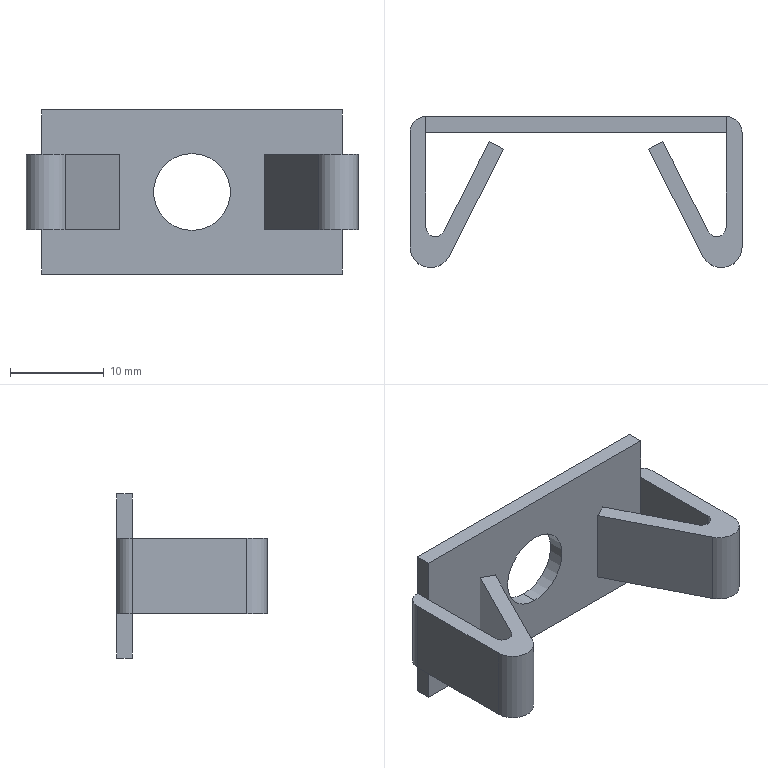Part | SolidWorks | features BaseBody 1 | 1 solid | 30 faces | box 35.4 x 16.108 x 17.5 mm | volume 1712 mm3 | plane 22 | cylinder 8 | commonest cylinder face diameters 2 x2 3.4 x2 4.4 x2 8.2 x2
STEP:
#1=CARTESIAN_POINT('',(0.,-1.7,-4.1));
#2=VERTEX_POINT('',#1);
#3=CARTESIAN_POINT('',(0.,-1.7,4.1));
#4=VERTEX_POINT('',#3);
#5=CARTESIAN_POINT('',(0.,-1.7,0.));
#6=DIRECTION('',(0.,1.,0.));
#7=DIRECTION('',(0.,0.,1.));
#8=AXIS2_PLACEMENT_3D('',#5,#6,#7);
#9=CIRCLE('',#8,4.1);
#10=EDGE_CURVE('',#2,#4,#9,.T.);
#11=ORIENTED_EDGE('',*,*,#10,.F.);
#12=CARTESIAN_POINT('',(0.,0.,-4.1));
#13=VERTEX_POINT('',#12);
#14=CARTESIAN_POINT('',(0.,-1.7,-4.1));
#15=DIRECTION('',(0.,1.,0.));
#16=VECTOR('',#15,1000.);
#17=LINE('',#14,#16);
#18=EDGE_CURVE('',#2,#13,#17,.T.);
#19=ORIENTED_EDGE('',*,*,#18,.T.);
#20=CARTESIAN_POINT('',(0.,0.,4.1));
#21=VERTEX_POINT('',#20);
#22=CARTESIAN_POINT('',(0.,0.,0.));
#23=DIRECTION('',(0.,1.,0.));
#24=DIRECTION('',(0.,0.,1.));
#25=AXIS2_PLACEMENT_3D('',#22,#23,#24);
#26=CIRCLE('',#25,4.1);
#27=EDGE_CURVE('',#13,#21,#26,.T.);
#28=ORIENTED_EDGE('',*,*,#27,.T.);
#29=CARTESIAN_POINT('',(0.,-1.7,4.1));
#30=DIRECTION('',(0.,1.,0.));
#31=VECTOR('',#30,1000.);
#32=LINE('',#29,#31);
#33=EDGE_CURVE('',#4,#21,#32,.T.);
#34=ORIENTED_EDGE('',*,*,#33,.F.);
#35=EDGE_LOOP('',(#11,#19,#28,#34));
#36=FACE_OUTER_BOUND('',#35,.T.);
#37=CARTESIAN_POINT('',(0.,-1.7,0.));
#38=DIRECTION('',(0.,1.,0.));
#39=DIRECTION('',(0.,0.,1.));
#40=AXIS2_PLACEMENT_3D('',#37,#38,#39);
#41=CYLINDRICAL_SURFACE('',#40,4.1);
#42=ADVANCED_FACE('',(#36),#41,.F.);
#43=CARTESIAN_POINT('',(-16.,0.,-4.));
#44=VERTEX_POINT('',#43);
#45=CARTESIAN_POINT('',(-16.,0.,-8.75));
#46=VERTEX_POINT('',#45);
#47=CARTESIAN_POINT('',(-16.,0.,8.75));
#48=DIRECTION('',(0.,0.,-1.));
#49=VECTOR('',#48,1000.);
#50=LINE('',#47,#49);
#51=EDGE_CURVE('',#44,#46,#50,.T.);
#52=ORIENTED_EDGE('',*,*,#51,.F.);
#53=CARTESIAN_POINT('',(-16.,0.,4.));
#54=VERTEX_POINT('',#53);
#55=CARTESIAN_POINT('',(-16.,0.,8.75));
#56=DIRECTION('',(0.,0.,-1.));
#57=VECTOR('',#56,1000.);
#58=LINE('',#55,#57);
#59=EDGE_CURVE('',#54,#44,#58,.T.);
#60=ORIENTED_EDGE('',*,*,#59,.F.);
#61=CARTESIAN_POINT('',(-16.,0.,8.75));
#62=VERTEX_POINT('',#61);
#63=CARTESIAN_POINT('',(-16.,0.,8.75));
#64=DIRECTION('',(0.,0.,-1.));
#65=VECTOR('',#64,1000.);
#66=LINE('',#63,#65);
#67=EDGE_CURVE('',#62,#54,#66,.T.);
#68=ORIENTED_EDGE('',*,*,#67,.F.);
#69=CARTESIAN_POINT('',(16.,0.,8.75));
#70=VERTEX_POINT('',#69);
#71=CARTESIAN_POINT('',(16.,0.,8.75));
#72=DIRECTION('',(-1.,0.,0.));
#73=VECTOR('',#72,1000.);
#74=LINE('',#71,#73);
#75=EDGE_CURVE('',#70,#62,#74,.T.);
#76=ORIENTED_EDGE('',*,*,#75,.F.);
#77=CARTESIAN_POINT('',(16.,0.,4.));
#78=VERTEX_POINT('',#77);
#79=CARTESIAN_POINT('',(16.,0.,8.75));
#80=DIRECTION('',(0.,0.,1.));
#81=VECTOR('',#80,1000.);
#82=LINE('',#79,#81);
#83=EDGE_CURVE('',#78,#70,#82,.T.);
#84=ORIENTED_EDGE('',*,*,#83,.F.);
#85=CARTESIAN_POINT('',(16.,0.,-4.));
#86=VERTEX_POINT('',#85);
#87=CARTESIAN_POINT('',(16.,0.,8.75));
#88=DIRECTION('',(0.,0.,1.));
#89=VECTOR('',#88,1000.);
#90=LINE('',#87,#89);
#91=EDGE_CURVE('',#86,#78,#90,.T.);
#92=ORIENTED_EDGE('',*,*,#91,.F.);
#93=CARTESIAN_POINT('',(16.,0.,-8.75));
#94=VERTEX_POINT('',#93);
#95=CARTESIAN_POINT('',(16.,0.,8.75));
#96=DIRECTION('',(0.,0.,1.));
#97=VECTOR('',#96,1000.);
#98=LINE('',#95,#97);
#99=EDGE_CURVE('',#94,#86,#98,.T.);
#100=ORIENTED_EDGE('',*,*,#99,.F.);
#101=CARTESIAN_POINT('',(16.,0.,-8.75));
#102=DIRECTION('',(1.,0.,0.));
#103=VECTOR('',#102,1000.);
#104=LINE('',#101,#103);
#105=EDGE_CURVE('',#46,#94,#104,.T.);
#106=ORIENTED_EDGE('',*,*,#105,.F.);
#107=EDGE_LOOP('',(#52,#60,#68,#76,#84,#92,#100,#106));
#108=FACE_OUTER_BOUND('',#107,.T.);
#109=CARTESIAN_POINT('',(0.,0.,0.));
#110=DIRECTION('',(0.,1.,0.));
#111=DIRECTION('',(0.,0.,1.));
#112=AXIS2_PLACEMENT_3D('',#109,#110,#111);
#113=CIRCLE('',#112,4.1);
#114=EDGE_CURVE('',#21,#13,#113,.T.);
#115=ORIENTED_EDGE('',*,*,#114,.F.);
#116=ORIENTED_EDGE('',*,*,#27,.F.);
#117=EDGE_LOOP('',(#115,#116));
#118=FACE_BOUND('',#117,.T.);
#119=CARTESIAN_POINT('',(16.,0.,8.75));
#120=DIRECTION('',(0.,-1.,0.));
#121=DIRECTION('',(0.,0.,-1.));
#122=AXIS2_PLACEMENT_3D('',#119,#120,#121);
#123=PLANE('',#122);
#124=ADVANCED_FACE('',(#108,#118),#123,.F.);
#125=ORIENTED_EDGE('',*,*,#105,.T.);
#126=CARTESIAN_POINT('',(16.,-1.7,-8.75));
#127=VERTEX_POINT('',#126);
#128=CARTESIAN_POINT('',(16.,0.,-8.75));
#129=DIRECTION('',(0.,1.,0.));
#130=VECTOR('',#129,1000.);
#131=LINE('',#128,#130);
#132=EDGE_CURVE('',#127,#94,#131,.T.);
#133=ORIENTED_EDGE('',*,*,#132,.F.);
#134=CARTESIAN_POINT('',(-16.,-1.7,-8.75));
#135=VERTEX_POINT('',#134);
#136=CARTESIAN_POINT('',(0.,-1.7,-8.75));
#137=DIRECTION('',(1.,0.,0.));
#138=VECTOR('',#137,1000.);
#139=LINE('',#136,#138);
#140=EDGE_CURVE('',#135,#127,#139,.T.);
#141=ORIENTED_EDGE('',*,*,#140,.F.);
#142=CARTESIAN_POINT('',(-16.,0.,-8.75));
#143=DIRECTION('',(0.,-1.,0.));
#144=VECTOR('',#143,1000.);
#145=LINE('',#142,#144);
#146=EDGE_CURVE('',#46,#135,#145,.T.);
#147=ORIENTED_EDGE('',*,*,#146,.F.);
#148=EDGE_LOOP('',(#125,#133,#141,#147));
#149=FACE_OUTER_BOUND('',#148,.T.);
#150=CARTESIAN_POINT('',(0.,0.,-8.75));
#151=DIRECTION('',(0.,0.,1.));
#152=DIRECTION('',(1.,0.,0.));
#153=AXIS2_PLACEMENT_3D('',#150,#151,#152);
#154=PLANE('',#153);
#155=ADVANCED_FACE('',(#149),#154,.F.);
#156=ORIENTED_EDGE('',*,*,#51,.T.);
#157=ORIENTED_EDGE('',*,*,#146,.T.);
#158=CARTESIAN_POINT('',(-16.,-1.7,-4.));
#159=VERTEX_POINT('',#158);
#160=CARTESIAN_POINT('',(-16.,-1.7,8.75));
#161=DIRECTION('',(0.,0.,-1.));
#162=VECTOR('',#161,1000.);
#163=LINE('',#160,#162);
#164=EDGE_CURVE('',#159,#135,#163,.T.);
#165=ORIENTED_EDGE('',*,*,#164,.F.);
#166=CARTESIAN_POINT('',(-16.,-1.7,-4.));
#167=DIRECTION('',(0.,1.,0.));
#168=VECTOR('',#167,1000.);
#169=LINE('',#166,#168);
#170=EDGE_CURVE('',#159,#44,#169,.T.);
#171=ORIENTED_EDGE('',*,*,#170,.T.);
#172=EDGE_LOOP('',(#156,#157,#165,#171));
#173=FACE_OUTER_BOUND('',#172,.T.);
#174=CARTESIAN_POINT('',(-16.,0.,8.75));
#175=DIRECTION('',(1.,0.,0.));
#176=DIRECTION('',(0.,0.,-1.));
#177=AXIS2_PLACEMENT_3D('',#174,#175,#176);
#178=PLANE('',#177);
#179=ADVANCED_FACE('',(#173),#178,.F.);
#180=CARTESIAN_POINT('',(-17.7,-1.7,4.));
#181=VERTEX_POINT('',#180);
#182=CARTESIAN_POINT('',(-16.,-1.7,4.));
#183=DIRECTION('',(0.,0.,-1.));
#184=DIRECTION('',(1.,0.,0.));
#185=AXIS2_PLACEMENT_3D('',#182,#183,#184);
#186=CIRCLE('',#185,1.7);
#187=EDGE_CURVE('',#181,#54,#186,.T.);
#188=ORIENTED_EDGE('',*,*,#187,.T.);
#189=ORIENTED_EDGE('',*,*,#59,.T.);
#190=CARTESIAN_POINT('',(-17.7,-1.7,-4.));
#191=VERTEX_POINT('',#190);
#192=CARTESIAN_POINT('',(-16.,-1.7,-4.));
#193=DIRECTION('',(0.,0.,1.));
#194=DIRECTION('',(1.,0.,0.));
#195=AXIS2_PLACEMENT_3D('',#192,#193,#194);
#196=CIRCLE('',#195,1.7);
#197=EDGE_CURVE('',#44,#191,#196,.T.);
#198=ORIENTED_EDGE('',*,*,#197,.T.);
#199=CARTESIAN_POINT('',(-17.7,-1.7,4.));
#200=DIRECTION('',(0.,0.,1.));
#201=VECTOR('',#200,1000.);
#202=LINE('',#199,#201);
#203=EDGE_CURVE('',#191,#181,#202,.T.);
#204=ORIENTED_EDGE('',*,*,#203,.T.);
#205=EDGE_LOOP('',(#188,#189,#198,#204));
#206=FACE_OUTER_BOUND('',#205,.T.);
#207=CARTESIAN_POINT('',(-16.,-1.7,4.));
#208=DIRECTION('',(0.,0.,1.));
#209=DIRECTION('',(1.,0.,0.));
#210=AXIS2_PLACEMENT_3D('',#207,#208,#209);
#211=CYLINDRICAL_SURFACE('',#210,1.7);
#212=ADVANCED_FACE('',(#206),#211,.T.);
#213=CARTESIAN_POINT('',(-16.,-1.7,4.));
#214=VERTEX_POINT('',#213);
#215=CARTESIAN_POINT('',(-16.,0.,4.));
#216=DIRECTION('',(0.,1.,0.));
#217=VECTOR('',#216,1000.);
#218=LINE('',#215,#217);
#219=EDGE_CURVE('',#214,#54,#218,.T.);
#220=ORIENTED_EDGE('',*,*,#219,.F.);
#221=CARTESIAN_POINT('',(-16.,-1.7,8.75));
#222=VERTEX_POINT('',#221);
#223=CARTESIAN_POINT('',(-16.,-1.7,8.75));
#224=DIRECTION('',(0.,0.,-1.));
#225=VECTOR('',#224,1000.);
#226=LINE('',#223,#225);
#227=EDGE_CURVE('',#222,#214,#226,.T.);
#228=ORIENTED_EDGE('',*,*,#227,.F.);
#229=CARTESIAN_POINT('',(-16.,0.,8.75));
#230=DIRECTION('',(0.,-1.,0.));
#231=VECTOR('',#230,1000.);
#232=LINE('',#229,#231);
#233=EDGE_CURVE('',#62,#222,#232,.T.);
#234=ORIENTED_EDGE('',*,*,#233,.F.);
#235=ORIENTED_EDGE('',*,*,#67,.T.);
#236=EDGE_LOOP('',(#220,#228,#234,#235));
#237=FACE_OUTER_BOUND('',#236,.T.);
#238=CARTESIAN_POINT('',(-16.,0.,8.75));
#239=DIRECTION('',(1.,0.,0.));
#240=DIRECTION('',(0.,0.,-1.));
#241=AXIS2_PLACEMENT_3D('',#238,#239,#240);
#242=PLANE('',#241);
#243=ADVANCED_FACE('',(#237),#242,.F.);
#244=CARTESIAN_POINT('',(16.,-1.7,8.75));
#245=VERTEX_POINT('',#244);
#246=CARTESIAN_POINT('',(16.,0.,8.75));
#247=DIRECTION('',(0.,1.,0.));
#248=VECTOR('',#247,1000.);
#249=LINE('',#246,#248);
#250=EDGE_CURVE('',#245,#70,#249,.T.);
#251=ORIENTED_EDGE('',*,*,#250,.T.);
#252=ORIENTED_EDGE('',*,*,#75,.T.);
#253=ORIENTED_EDGE('',*,*,#233,.T.);
#254=CARTESIAN_POINT('',(0.,-1.7,8.75));
#255=DIRECTION('',(1.,0.,0.));
#256=VECTOR('',#255,1000.);
#257=LINE('',#254,#256);
#258=EDGE_CURVE('',#222,#245,#257,.T.);
#259=ORIENTED_EDGE('',*,*,#258,.T.);
#260=EDGE_LOOP('',(#251,#252,#253,#259));
#261=FACE_OUTER_BOUND('',#260,.T.);
#262=CARTESIAN_POINT('',(0.,0.,8.75));
#263=DIRECTION('',(0.,0.,1.));
#264=DIRECTION('',(1.,0.,0.));
#265=AXIS2_PLACEMENT_3D('',#262,#263,#264);
#266=PLANE('',#265);
#267=ADVANCED_FACE('',(#261),#266,.T.);
#268=CARTESIAN_POINT('',(16.,-1.7,4.));
#269=VERTEX_POINT('',#268);
#270=CARTESIAN_POINT('',(16.,-13.908,4.));
#271=DIRECTION('',(0.,-1.,0.));
#272=VECTOR('',#271,1000.);
#273=LINE('',#270,#272);
#274=EDGE_CURVE('',#78,#269,#273,.T.);
#275=ORIENTED_EDGE('',*,*,#274,.F.);
#276=ORIENTED_EDGE('',*,*,#83,.T.);
#277=ORIENTED_EDGE('',*,*,#250,.F.);
#278=CARTESIAN_POINT('',(16.,-1.7,8.75));
#279=DIRECTION('',(0.,0.,1.));
#280=VECTOR('',#279,1000.);
#281=LINE('',#278,#280);
#282=EDGE_CURVE('',#269,#245,#281,.T.);
#283=ORIENTED_EDGE('',*,*,#282,.F.);
#284=EDGE_LOOP('',(#275,#276,#277,#283));
#285=FACE_OUTER_BOUND('',#284,.T.);
#286=CARTESIAN_POINT('',(16.,-1.7,8.75));
#287=DIRECTION('',(-1.,0.,0.));
#288=DIRECTION('',(0.,0.,1.));
#289=AXIS2_PLACEMENT_3D('',#286,#287,#288);
#290=PLANE('',#289);
#291=ADVANCED_FACE('',(#285),#290,.F.);
#292=CARTESIAN_POINT('',(17.7,-1.7,4.));
#293=VERTEX_POINT('',#292);
#294=CARTESIAN_POINT('',(16.,-1.7,4.));
#295=DIRECTION('',(0.,0.,-1.));
#296=DIRECTION('',(1.,0.,0.));
#297=AXIS2_PLACEMENT_3D('',#294,#295,#296);
#298=CIRCLE('',#297,1.7);
#299=EDGE_CURVE('',#78,#293,#298,.T.);
#300=ORIENTED_EDGE('',*,*,#299,.T.);
#301=CARTESIAN_POINT('',(17.7,-1.7,-4.));
#302=VERTEX_POINT('',#301);
#303=CARTESIAN_POINT('',(17.7,-1.7,4.));
#304=DIRECTION('',(0.,0.,-1.));
#305=VECTOR('',#304,1000.);
#306=LINE('',#303,#305);
#307=EDGE_CURVE('',#293,#302,#306,.T.);
#308=ORIENTED_EDGE('',*,*,#307,.T.);
#309=CARTESIAN_POINT('',(16.,-1.7,-4.));
#310=DIRECTION('',(0.,0.,1.));
#311=DIRECTION('',(1.,0.,0.));
#312=AXIS2_PLACEMENT_3D('',#309,#310,#311);
#313=CIRCLE('',#312,1.7);
#314=EDGE_CURVE('',#302,#86,#313,.T.);
#315=ORIENTED_EDGE('',*,*,#314,.T.);
#316=ORIENTED_EDGE('',*,*,#91,.T.);
#317=EDGE_LOOP('',(#300,#308,#315,#316));
#318=FACE_OUTER_BOUND('',#317,.T.);
#319=CARTESIAN_POINT('',(16.,-1.7,4.));
#320=DIRECTION('',(0.,0.,1.));
#321=DIRECTION('',(1.,0.,0.));
#322=AXIS2_PLACEMENT_3D('',#319,#320,#321);
#323=CYLINDRICAL_SURFACE('',#322,1.7);
#324=ADVANCED_FACE('',(#318),#323,.T.);
#325=CARTESIAN_POINT('',(16.,-1.7,-4.));
#326=VERTEX_POINT('',#325);
#327=CARTESIAN_POINT('',(16.,-1.7,8.75));
#328=DIRECTION('',(0.,0.,1.));
#329=VECTOR('',#328,1000.);
#330=LINE('',#327,#329);
#331=EDGE_CURVE('',#127,#326,#330,.T.);
#332=ORIENTED_EDGE('',*,*,#331,.F.);
#333=ORIENTED_EDGE('',*,*,#132,.T.);
#334=ORIENTED_EDGE('',*,*,#99,.T.);
#335=CARTESIAN_POINT('',(16.,-1.7,-4.));
#336=DIRECTION('',(0.,1.,0.));
#337=VECTOR('',#336,1000.);
#338=LINE('',#335,#337);
#339=EDGE_CURVE('',#326,#86,#338,.T.);
#340=ORIENTED_EDGE('',*,*,#339,.F.);
#341=EDGE_LOOP('',(#332,#333,#334,#340));
#342=FACE_OUTER_BOUND('',#341,.T.);
#343=CARTESIAN_POINT('',(16.,-1.7,8.75));
#344=DIRECTION('',(-1.,0.,0.));
#345=DIRECTION('',(0.,0.,1.));
#346=AXIS2_PLACEMENT_3D('',#343,#344,#345);
#347=PLANE('',#346);
#348=ADVANCED_FACE('',(#342),#347,.F.);
#349=ORIENTED_EDGE('',*,*,#18,.F.);
#350=CARTESIAN_POINT('',(0.,-1.7,0.));
#351=DIRECTION('',(0.,1.,0.));
#352=DIRECTION('',(0.,0.,1.));
#353=AXIS2_PLACEMENT_3D('',#350,#351,#352);
#354=CIRCLE('',#353,4.1);
#355=EDGE_CURVE('',#4,#2,#354,.T.);
#356=ORIENTED_EDGE('',*,*,#355,.F.);
#357=ORIENTED_EDGE('',*,*,#33,.T.);
#358=ORIENTED_EDGE('',*,*,#114,.T.);
#359=EDGE_LOOP('',(#349,#356,#357,#358));
#360=FACE_OUTER_BOUND('',#359,.T.);
#361=CARTESIAN_POINT('',(0.,-1.7,0.));
#362=DIRECTION('',(0.,1.,0.));
#363=DIRECTION('',(0.,0.,1.));
#364=AXIS2_PLACEMENT_3D('',#361,#362,#363);
#365=CYLINDRICAL_SURFACE('',#364,4.1);
#366=ADVANCED_FACE('',(#360),#365,.F.);
#367=ORIENTED_EDGE('',*,*,#331,.T.);
#368=CARTESIAN_POINT('',(16.,-1.7,8.75));
#369=DIRECTION('',(0.,0.,-1.));
#370=VECTOR('',#369,1000.);
#371=LINE('',#368,#370);
#372=EDGE_CURVE('',#269,#326,#371,.T.);
#373=ORIENTED_EDGE('',*,*,#372,.F.);
#374=ORIENTED_EDGE('',*,*,#282,.T.);
#375=ORIENTED_EDGE('',*,*,#258,.F.);
#376=ORIENTED_EDGE('',*,*,#227,.T.);
#377=CARTESIAN_POINT('',(-16.,-1.7,8.75));
#378=DIRECTION('',(0.,0.,1.));
#379=VECTOR('',#378,1000.);
#380=LINE('',#377,#379);
#381=EDGE_CURVE('',#159,#214,#380,.T.);
#382=ORIENTED_EDGE('',*,*,#381,.F.);
#383=ORIENTED_EDGE('',*,*,#164,.T.);
#384=ORIENTED_EDGE('',*,*,#140,.T.);
#385=EDGE_LOOP('',(#367,#373,#374,#375,#376,#382,#383,#384));
#386=FACE_OUTER_BOUND('',#385,.T.);
#387=ORIENTED_EDGE('',*,*,#355,.T.);
#388=ORIENTED_EDGE('',*,*,#10,.T.);
#389=EDGE_LOOP('',(#387,#388));
#390=FACE_BOUND('',#389,.T.);
#391=CARTESIAN_POINT('',(-16.,-1.7,8.75));
#392=DIRECTION('',(0.,1.,0.));
#393=DIRECTION('',(0.,0.,1.));
#394=AXIS2_PLACEMENT_3D('',#391,#392,#393);
#395=PLANE('',#394);
#396=ADVANCED_FACE('',(#386,#390),#395,.F.);
#397=CARTESIAN_POINT('',(-16.,-11.816,4.));
#398=VERTEX_POINT('',#397);
#399=CARTESIAN_POINT('',(-16.,-1.7,4.));
#400=DIRECTION('',(0.,1.,0.));
#401=VECTOR('',#400,1000.);
#402=LINE('',#399,#401);
#403=EDGE_CURVE('',#398,#214,#402,.T.);
#404=ORIENTED_EDGE('',*,*,#403,.T.);
#405=ORIENTED_EDGE('',*,*,#219,.T.);
#406=ORIENTED_EDGE('',*,*,#187,.F.);
#407=CARTESIAN_POINT('',(-17.7,-13.908,4.));
#408=VERTEX_POINT('',#407);
#409=CARTESIAN_POINT('',(-17.7,-1.7,4.));
#410=DIRECTION('',(0.,-1.,0.));
#411=VECTOR('',#410,1000.);
#412=LINE('',#409,#411);
#413=EDGE_CURVE('',#181,#408,#412,.T.);
#414=ORIENTED_EDGE('',*,*,#413,.T.);
#415=CARTESIAN_POINT('',(-13.538,-14.903,4.));
#416=VERTEX_POINT('',#415);
#417=CARTESIAN_POINT('',(-15.5,-13.908,4.));
#418=DIRECTION('',(0.,0.,1.));
#419=DIRECTION('',(1.,0.,0.));
#420=AXIS2_PLACEMENT_3D('',#417,#418,#419);
#421=CIRCLE('',#420,2.2);
#422=EDGE_CURVE('',#408,#416,#421,.T.);
#423=ORIENTED_EDGE('',*,*,#422,.T.);
#424=CARTESIAN_POINT('',(-7.741,-3.469,4.));
#425=VERTEX_POINT('',#424);
#426=CARTESIAN_POINT('',(-13.538,-14.903,4.));
#427=DIRECTION('',(0.4522,0.8919,0.));
#428=VECTOR('',#427,1000.);
#429=LINE('',#426,#428);
#430=EDGE_CURVE('',#416,#425,#429,.T.);
#431=ORIENTED_EDGE('',*,*,#430,.T.);
#432=CARTESIAN_POINT('',(-9.257,-2.7,4.));
#433=VERTEX_POINT('',#432);
#434=CARTESIAN_POINT('',(-7.741,-3.469,4.));
#435=DIRECTION('',(-0.8919,0.4522,0.));
#436=VECTOR('',#435,1000.);
#437=LINE('',#434,#436);
#438=EDGE_CURVE('',#425,#433,#437,.T.);
#439=ORIENTED_EDGE('',*,*,#438,.T.);
#440=CARTESIAN_POINT('',(-14.108,-12.268,4.));
#441=VERTEX_POINT('',#440);
#442=CARTESIAN_POINT('',(-9.257,-2.7,4.));
#443=DIRECTION('',(-0.4522,-0.8919,0.));
#444=VECTOR('',#443,1000.);
#445=LINE('',#442,#444);
#446=EDGE_CURVE('',#433,#441,#445,.T.);
#447=ORIENTED_EDGE('',*,*,#446,.T.);
#448=CARTESIAN_POINT('',(-15.,-11.816,4.));
#449=DIRECTION('',(0.,0.,-1.));
#450=DIRECTION('',(1.,0.,0.));
#451=AXIS2_PLACEMENT_3D('',#448,#449,#450);
#452=CIRCLE('',#451,1.);
#453=EDGE_CURVE('',#441,#398,#452,.T.);
#454=ORIENTED_EDGE('',*,*,#453,.T.);
#455=EDGE_LOOP('',(#404,#405,#406,#414,#423,#431,#439,#447,#454));
#456=FACE_OUTER_BOUND('',#455,.T.);
#457=CARTESIAN_POINT('',(-16.,-1.7,4.));
#458=DIRECTION('',(0.,0.,1.));
#459=DIRECTION('',(1.,0.,0.));
#460=AXIS2_PLACEMENT_3D('',#457,#458,#459);
#461=PLANE('',#460);
#462=ADVANCED_FACE('',(#456),#461,.T.);
#463=CARTESIAN_POINT('',(-17.7,-13.908,-4.));
#464=VERTEX_POINT('',#463);
#465=CARTESIAN_POINT('',(-17.7,-13.908,4.));
#466=DIRECTION('',(0.,0.,-1.));
#467=VECTOR('',#466,1000.);
#468=LINE('',#465,#467);
#469=EDGE_CURVE('',#408,#464,#468,.T.);
#470=ORIENTED_EDGE('',*,*,#469,.F.);
#471=ORIENTED_EDGE('',*,*,#413,.F.);
#472=ORIENTED_EDGE('',*,*,#203,.F.);
#473=CARTESIAN_POINT('',(-17.7,-1.7,-4.));
#474=DIRECTION('',(0.,1.,0.));
#475=VECTOR('',#474,1000.);
#476=LINE('',#473,#475);
#477=EDGE_CURVE('',#464,#191,#476,.T.);
#478=ORIENTED_EDGE('',*,*,#477,.F.);
#479=EDGE_LOOP('',(#470,#471,#472,#478));
#480=FACE_OUTER_BOUND('',#479,.T.);
#481=CARTESIAN_POINT('',(-17.7,-1.7,4.));
#482=DIRECTION('',(1.,0.,0.));
#483=DIRECTION('',(0.,0.,-1.));
#484=AXIS2_PLACEMENT_3D('',#481,#482,#483);
#485=PLANE('',#484);
#486=ADVANCED_FACE('',(#480),#485,.F.);
#487=ORIENTED_EDGE('',*,*,#170,.F.);
#488=CARTESIAN_POINT('',(-16.,-11.816,-4.));
#489=VERTEX_POINT('',#488);
#490=CARTESIAN_POINT('',(-16.,-1.7,-4.));
#491=DIRECTION('',(0.,1.,0.));
#492=VECTOR('',#491,1000.);
#493=LINE('',#490,#492);
#494=EDGE_CURVE('',#489,#159,#493,.T.);
#495=ORIENTED_EDGE('',*,*,#494,.F.);
#496=CARTESIAN_POINT('',(-14.108,-12.268,-4.));
#497=VERTEX_POINT('',#496);
#498=CARTESIAN_POINT('',(-15.,-11.816,-4.));
#499=DIRECTION('',(0.,0.,-1.));
#500=DIRECTION('',(1.,0.,0.));
#501=AXIS2_PLACEMENT_3D('',#498,#499,#500);
#502=CIRCLE('',#501,1.);
#503=EDGE_CURVE('',#497,#489,#502,.T.);
#504=ORIENTED_EDGE('',*,*,#503,.F.);
#505=CARTESIAN_POINT('',(-9.257,-2.7,-4.));
#506=VERTEX_POINT('',#505);
#507=CARTESIAN_POINT('',(-9.257,-2.7,-4.));
#508=DIRECTION('',(-0.4522,-0.8919,0.));
#509=VECTOR('',#508,1000.);
#510=LINE('',#507,#509);
#511=EDGE_CURVE('',#506,#497,#510,.T.);
#512=ORIENTED_EDGE('',*,*,#511,.F.);
#513=CARTESIAN_POINT('',(-7.741,-3.469,-4.));
#514=VERTEX_POINT('',#513);
#515=CARTESIAN_POINT('',(-7.741,-3.469,-4.));
#516=DIRECTION('',(0.8919,-0.4522,0.));
#517=VECTOR('',#516,1000.);
#518=LINE('',#515,#517);
#519=EDGE_CURVE('',#506,#514,#518,.T.);
#520=ORIENTED_EDGE('',*,*,#519,.T.);
#521=CARTESIAN_POINT('',(-13.538,-14.903,-4.));
#522=VERTEX_POINT('',#521);
#523=CARTESIAN_POINT('',(-13.538,-14.903,-4.));
#524=DIRECTION('',(0.4522,0.8919,0.));
#525=VECTOR('',#524,1000.);
#526=LINE('',#523,#525);
#527=EDGE_CURVE('',#522,#514,#526,.T.);
#528=ORIENTED_EDGE('',*,*,#527,.F.);
#529=CARTESIAN_POINT('',(-15.5,-13.908,-4.));
#530=DIRECTION('',(0.,0.,1.));
#531=DIRECTION('',(1.,0.,0.));
#532=AXIS2_PLACEMENT_3D('',#529,#530,#531);
#533=CIRCLE('',#532,2.2);
#534=EDGE_CURVE('',#464,#522,#533,.T.);
#535=ORIENTED_EDGE('',*,*,#534,.F.);
#536=ORIENTED_EDGE('',*,*,#477,.T.);
#537=ORIENTED_EDGE('',*,*,#197,.F.);
#538=EDGE_LOOP('',(#487,#495,#504,#512,#520,#528,#535,#536,#537));
#539=FACE_OUTER_BOUND('',#538,.T.);
#540=CARTESIAN_POINT('',(-16.,-1.7,-4.));
#541=DIRECTION('',(0.,0.,1.));
#542=DIRECTION('',(1.,0.,0.));
#543=AXIS2_PLACEMENT_3D('',#540,#541,#542);
#544=PLANE('',#543);
#545=ADVANCED_FACE('',(#539),#544,.F.);
#546=ORIENTED_EDGE('',*,*,#307,.F.);
#547=CARTESIAN_POINT('',(17.7,-13.908,4.));
#548=VERTEX_POINT('',#547);
#549=CARTESIAN_POINT('',(17.7,-13.908,4.));
#550=DIRECTION('',(0.,1.,0.));
#551=VECTOR('',#550,1000.);
#552=LINE('',#549,#551);
#553=EDGE_CURVE('',#548,#293,#552,.T.);
#554=ORIENTED_EDGE('',*,*,#553,.F.);
#555=CARTESIAN_POINT('',(17.7,-13.908,-4.));
#556=VERTEX_POINT('',#555);
#557=CARTESIAN_POINT('',(17.7,-13.908,4.));
#558=DIRECTION('',(0.,0.,1.));
#559=VECTOR('',#558,1000.);
#560=LINE('',#557,#559);
#561=EDGE_CURVE('',#556,#548,#560,.T.);
#562=ORIENTED_EDGE('',*,*,#561,.F.);
#563=CARTESIAN_POINT('',(17.7,-13.908,-4.));
#564=DIRECTION('',(0.,-1.,0.));
#565=VECTOR('',#564,1000.);
#566=LINE('',#563,#565);
#567=EDGE_CURVE('',#302,#556,#566,.T.);
#568=ORIENTED_EDGE('',*,*,#567,.F.);
#569=EDGE_LOOP('',(#546,#554,#562,#568));
#570=FACE_OUTER_BOUND('',#569,.T.);
#571=CARTESIAN_POINT('',(17.7,-13.908,4.));
#572=DIRECTION('',(-1.,0.,0.));
#573=DIRECTION('',(0.,0.,1.));
#574=AXIS2_PLACEMENT_3D('',#571,#572,#573);
#575=PLANE('',#574);
#576=ADVANCED_FACE('',(#570),#575,.F.);
#577=CARTESIAN_POINT('',(16.,-11.816,4.));
#578=VERTEX_POINT('',#577);
#579=CARTESIAN_POINT('',(14.108,-12.268,4.));
#580=VERTEX_POINT('',#579);
#581=CARTESIAN_POINT('',(15.,-11.816,4.));
#582=DIRECTION('',(0.,0.,-1.));
#583=DIRECTION('',(1.,0.,0.));
#584=AXIS2_PLACEMENT_3D('',#581,#582,#583);
#585=CIRCLE('',#584,1.);
#586=EDGE_CURVE('',#578,#580,#585,.T.);
#587=ORIENTED_EDGE('',*,*,#586,.T.);
#588=CARTESIAN_POINT('',(9.257,-2.7,4.));
#589=VERTEX_POINT('',#588);
#590=CARTESIAN_POINT('',(14.108,-12.268,4.));
#591=DIRECTION('',(-0.4522,0.8919,0.));
#592=VECTOR('',#591,1000.);
#593=LINE('',#590,#592);
#594=EDGE_CURVE('',#580,#589,#593,.T.);
#595=ORIENTED_EDGE('',*,*,#594,.T.);
#596=CARTESIAN_POINT('',(7.741,-3.469,4.));
#597=VERTEX_POINT('',#596);
#598=CARTESIAN_POINT('',(9.257,-2.7,4.));
#599=DIRECTION('',(-0.8919,-0.4522,0.));
#600=VECTOR('',#599,1000.);
#601=LINE('',#598,#600);
#602=EDGE_CURVE('',#589,#597,#601,.T.);
#603=ORIENTED_EDGE('',*,*,#602,.T.);
#604=CARTESIAN_POINT('',(13.538,-14.903,4.));
#605=VERTEX_POINT('',#604);
#606=CARTESIAN_POINT('',(7.741,-3.469,4.));
#607=DIRECTION('',(0.4522,-0.8919,0.));
#608=VECTOR('',#607,1000.);
#609=LINE('',#606,#608);
#610=EDGE_CURVE('',#597,#605,#609,.T.);
#611=ORIENTED_EDGE('',*,*,#610,.T.);
#612=CARTESIAN_POINT('',(15.5,-13.908,4.));
#613=DIRECTION('',(0.,0.,1.));
#614=DIRECTION('',(1.,0.,0.));
#615=AXIS2_PLACEMENT_3D('',#612,#613,#614);
#616=CIRCLE('',#615,2.2);
#617=EDGE_CURVE('',#605,#548,#616,.T.);
#618=ORIENTED_EDGE('',*,*,#617,.T.);
#619=ORIENTED_EDGE('',*,*,#553,.T.);
#620=ORIENTED_EDGE('',*,*,#299,.F.);
#621=ORIENTED_EDGE('',*,*,#274,.T.);
#622=CARTESIAN_POINT('',(16.,-13.908,4.));
#623=DIRECTION('',(0.,-1.,0.));
#624=VECTOR('',#623,1000.);
#625=LINE('',#622,#624);
#626=EDGE_CURVE('',#269,#578,#625,.T.);
#627=ORIENTED_EDGE('',*,*,#626,.T.);
#628=EDGE_LOOP('',(#587,#595,#603,#611,#618,#619,#620,#621,#627));
#629=FACE_OUTER_BOUND('',#628,.T.);
#630=CARTESIAN_POINT('',(15.5,-13.908,4.));
#631=DIRECTION('',(0.,0.,1.));
#632=DIRECTION('',(1.,0.,0.));
#633=AXIS2_PLACEMENT_3D('',#630,#631,#632);
#634=PLANE('',#633);
#635=ADVANCED_FACE('',(#629),#634,.T.);
#636=CARTESIAN_POINT('',(14.108,-12.268,-4.));
#637=VERTEX_POINT('',#636);
#638=CARTESIAN_POINT('',(9.257,-2.7,-4.));
#639=VERTEX_POINT('',#638);
#640=CARTESIAN_POINT('',(14.108,-12.268,-4.));
#641=DIRECTION('',(-0.4522,0.8919,0.));
#642=VECTOR('',#641,1000.);
#643=LINE('',#640,#642);
#644=EDGE_CURVE('',#637,#639,#643,.T.);
#645=ORIENTED_EDGE('',*,*,#644,.F.);
#646=CARTESIAN_POINT('',(16.,-11.816,-4.));
#647=VERTEX_POINT('',#646);
#648=CARTESIAN_POINT('',(15.,-11.816,-4.));
#649=DIRECTION('',(0.,0.,-1.));
#650=DIRECTION('',(1.,0.,0.));
#651=AXIS2_PLACEMENT_3D('',#648,#649,#650);
#652=CIRCLE('',#651,1.);
#653=EDGE_CURVE('',#647,#637,#652,.T.);
#654=ORIENTED_EDGE('',*,*,#653,.F.);
#655=CARTESIAN_POINT('',(16.,-13.908,-4.));
#656=DIRECTION('',(0.,-1.,0.));
#657=VECTOR('',#656,1000.);
#658=LINE('',#655,#657);
#659=EDGE_CURVE('',#326,#647,#658,.T.);
#660=ORIENTED_EDGE('',*,*,#659,.F.);
#661=ORIENTED_EDGE('',*,*,#339,.T.);
#662=ORIENTED_EDGE('',*,*,#314,.F.);
#663=ORIENTED_EDGE('',*,*,#567,.T.);
#664=CARTESIAN_POINT('',(13.538,-14.903,-4.));
#665=VERTEX_POINT('',#664);
#666=CARTESIAN_POINT('',(15.5,-13.908,-4.));
#667=DIRECTION('',(0.,0.,1.));
#668=DIRECTION('',(1.,0.,0.));
#669=AXIS2_PLACEMENT_3D('',#666,#667,#668);
#670=CIRCLE('',#669,2.2);
#671=EDGE_CURVE('',#665,#556,#670,.T.);
#672=ORIENTED_EDGE('',*,*,#671,.F.);
#673=CARTESIAN_POINT('',(7.741,-3.469,-4.));
#674=VERTEX_POINT('',#673);
#675=CARTESIAN_POINT('',(7.741,-3.469,-4.));
#676=DIRECTION('',(0.4522,-0.8919,0.));
#677=VECTOR('',#676,1000.);
#678=LINE('',#675,#677);
#679=EDGE_CURVE('',#674,#665,#678,.T.);
#680=ORIENTED_EDGE('',*,*,#679,.F.);
#681=CARTESIAN_POINT('',(9.257,-2.7,-4.));
#682=DIRECTION('',(0.8919,0.4522,0.));
#683=VECTOR('',#682,1000.);
#684=LINE('',#681,#683);
#685=EDGE_CURVE('',#674,#639,#684,.T.);
#686=ORIENTED_EDGE('',*,*,#685,.T.);
#687=EDGE_LOOP('',(#645,#654,#660,#661,#662,#663,#672,#680,#686));
#688=FACE_OUTER_BOUND('',#687,.T.);
#689=CARTESIAN_POINT('',(15.5,-13.908,-4.));
#690=DIRECTION('',(0.,0.,1.));
#691=DIRECTION('',(1.,0.,0.));
#692=AXIS2_PLACEMENT_3D('',#689,#690,#691);
#693=PLANE('',#692);
#694=ADVANCED_FACE('',(#688),#693,.F.);
#695=ORIENTED_EDGE('',*,*,#372,.T.);
#696=ORIENTED_EDGE('',*,*,#659,.T.);
#697=CARTESIAN_POINT('',(16.,-11.816,4.));
#698=DIRECTION('',(0.,0.,-1.));
#699=VECTOR('',#698,1000.);
#700=LINE('',#697,#699);
#701=EDGE_CURVE('',#578,#647,#700,.T.);
#702=ORIENTED_EDGE('',*,*,#701,.F.);
#703=ORIENTED_EDGE('',*,*,#626,.F.);
#704=EDGE_LOOP('',(#695,#696,#702,#703));
#705=FACE_OUTER_BOUND('',#704,.T.);
#706=CARTESIAN_POINT('',(16.,0.,4.));
#707=DIRECTION('',(1.,0.,0.));
#708=DIRECTION('',(0.,0.,-1.));
#709=AXIS2_PLACEMENT_3D('',#706,#707,#708);
#710=PLANE('',#709);
#711=ADVANCED_FACE('',(#705),#710,.F.);
#712=ORIENTED_EDGE('',*,*,#381,.T.);
#713=ORIENTED_EDGE('',*,*,#403,.F.);
#714=CARTESIAN_POINT('',(-16.,-11.816,4.));
#715=DIRECTION('',(0.,0.,1.));
#716=VECTOR('',#715,1000.);
#717=LINE('',#714,#716);
#718=EDGE_CURVE('',#489,#398,#717,.T.);
#719=ORIENTED_EDGE('',*,*,#718,.F.);
#720=ORIENTED_EDGE('',*,*,#494,.T.);
#721=EDGE_LOOP('',(#712,#713,#719,#720));
#722=FACE_OUTER_BOUND('',#721,.T.);
#723=CARTESIAN_POINT('',(-16.,-11.816,4.));
#724=DIRECTION('',(-1.,0.,0.));
#725=DIRECTION('',(0.,0.,1.));
#726=AXIS2_PLACEMENT_3D('',#723,#724,#725);
#727=PLANE('',#726);
#728=ADVANCED_FACE('',(#722),#727,.F.);
#729=ORIENTED_EDGE('',*,*,#718,.T.);
#730=ORIENTED_EDGE('',*,*,#453,.F.);
#731=CARTESIAN_POINT('',(-14.108,-12.268,4.));
#732=DIRECTION('',(0.,0.,1.));
#733=VECTOR('',#732,1000.);
#734=LINE('',#731,#733);
#735=EDGE_CURVE('',#497,#441,#734,.T.);
#736=ORIENTED_EDGE('',*,*,#735,.F.);
#737=ORIENTED_EDGE('',*,*,#503,.T.);
#738=EDGE_LOOP('',(#729,#730,#736,#737));
#739=FACE_OUTER_BOUND('',#738,.T.);
#740=CARTESIAN_POINT('',(-15.,-11.816,4.));
#741=DIRECTION('',(0.,0.,1.));
#742=DIRECTION('',(1.,0.,0.));
#743=AXIS2_PLACEMENT_3D('',#740,#741,#742);
#744=CYLINDRICAL_SURFACE('',#743,1.);
#745=ADVANCED_FACE('',(#739),#744,.F.);
#746=ORIENTED_EDGE('',*,*,#735,.T.);
#747=ORIENTED_EDGE('',*,*,#446,.F.);
#748=CARTESIAN_POINT('',(-9.257,-2.7,4.));
#749=DIRECTION('',(0.,0.,1.));
#750=VECTOR('',#749,1000.);
#751=LINE('',#748,#750);
#752=EDGE_CURVE('',#506,#433,#751,.T.);
#753=ORIENTED_EDGE('',*,*,#752,.F.);
#754=ORIENTED_EDGE('',*,*,#511,.T.);
#755=EDGE_LOOP('',(#746,#747,#753,#754));
#756=FACE_OUTER_BOUND('',#755,.T.);
#757=CARTESIAN_POINT('',(-9.257,-2.7,4.));
#758=DIRECTION('',(0.8919,-0.4522,0.));
#759=DIRECTION('',(0.4522,0.8919,0.));
#760=AXIS2_PLACEMENT_3D('',#757,#758,#759);
#761=PLANE('',#760);
#762=ADVANCED_FACE('',(#756),#761,.F.);
#763=CARTESIAN_POINT('',(-7.741,-3.469,4.));
#764=DIRECTION('',(0.,0.,-1.));
#765=VECTOR('',#764,1000.);
#766=LINE('',#763,#765);
#767=EDGE_CURVE('',#425,#514,#766,.T.);
#768=ORIENTED_EDGE('',*,*,#767,.F.);
#769=ORIENTED_EDGE('',*,*,#430,.F.);
#770=CARTESIAN_POINT('',(-13.538,-14.903,4.));
#771=DIRECTION('',(0.,0.,1.));
#772=VECTOR('',#771,1000.);
#773=LINE('',#770,#772);
#774=EDGE_CURVE('',#522,#416,#773,.T.);
#775=ORIENTED_EDGE('',*,*,#774,.F.);
#776=ORIENTED_EDGE('',*,*,#527,.T.);
#777=EDGE_LOOP('',(#768,#769,#775,#776));
#778=FACE_OUTER_BOUND('',#777,.T.);
#779=CARTESIAN_POINT('',(-13.538,-14.903,4.));
#780=DIRECTION('',(-0.8919,0.4522,0.));
#781=DIRECTION('',(-0.4522,-0.8919,0.));
#782=AXIS2_PLACEMENT_3D('',#779,#780,#781);
#783=PLANE('',#782);
#784=ADVANCED_FACE('',(#778),#783,.F.);
#785=ORIENTED_EDGE('',*,*,#422,.F.);
#786=ORIENTED_EDGE('',*,*,#469,.T.);
#787=ORIENTED_EDGE('',*,*,#534,.T.);
#788=ORIENTED_EDGE('',*,*,#774,.T.);
#789=EDGE_LOOP('',(#785,#786,#787,#788));
#790=FACE_OUTER_BOUND('',#789,.T.);
#791=CARTESIAN_POINT('',(-15.5,-13.908,4.));
#792=DIRECTION('',(0.,0.,1.));
#793=DIRECTION('',(1.,0.,0.));
#794=AXIS2_PLACEMENT_3D('',#791,#792,#793);
#795=CYLINDRICAL_SURFACE('',#794,2.2);
#796=ADVANCED_FACE('',(#790),#795,.T.);
#797=ORIENTED_EDGE('',*,*,#617,.F.);
#798=CARTESIAN_POINT('',(13.538,-14.903,4.));
#799=DIRECTION('',(0.,0.,-1.));
#800=VECTOR('',#799,1000.);
#801=LINE('',#798,#800);
#802=EDGE_CURVE('',#605,#665,#801,.T.);
#803=ORIENTED_EDGE('',*,*,#802,.T.);
#804=ORIENTED_EDGE('',*,*,#671,.T.);
#805=ORIENTED_EDGE('',*,*,#561,.T.);
#806=EDGE_LOOP('',(#797,#803,#804,#805));
#807=FACE_OUTER_BOUND('',#806,.T.);
#808=CARTESIAN_POINT('',(15.5,-13.908,4.));
#809=DIRECTION('',(0.,0.,1.));
#810=DIRECTION('',(1.,0.,0.));
#811=AXIS2_PLACEMENT_3D('',#808,#809,#810);
#812=CYLINDRICAL_SURFACE('',#811,2.2);
#813=ADVANCED_FACE('',(#807),#812,.T.);
#814=CARTESIAN_POINT('',(9.257,-2.7,4.));
#815=DIRECTION('',(0.,0.,-1.));
#816=VECTOR('',#815,1000.);
#817=LINE('',#814,#816);
#818=EDGE_CURVE('',#589,#639,#817,.T.);
#819=ORIENTED_EDGE('',*,*,#818,.F.);
#820=ORIENTED_EDGE('',*,*,#594,.F.);
#821=CARTESIAN_POINT('',(14.108,-12.268,4.));
#822=DIRECTION('',(0.,0.,1.));
#823=VECTOR('',#822,1000.);
#824=LINE('',#821,#823);
#825=EDGE_CURVE('',#637,#580,#824,.T.);
#826=ORIENTED_EDGE('',*,*,#825,.F.);
#827=ORIENTED_EDGE('',*,*,#644,.T.);
#828=EDGE_LOOP('',(#819,#820,#826,#827));
#829=FACE_OUTER_BOUND('',#828,.T.);
#830=CARTESIAN_POINT('',(14.108,-12.268,4.));
#831=DIRECTION('',(-0.8919,-0.4522,0.));
#832=DIRECTION('',(0.4522,-0.8919,0.));
#833=AXIS2_PLACEMENT_3D('',#830,#831,#832);
#834=PLANE('',#833);
#835=ADVANCED_FACE('',(#829),#834,.F.);
#836=ORIENTED_EDGE('',*,*,#825,.T.);
#837=ORIENTED_EDGE('',*,*,#586,.F.);
#838=ORIENTED_EDGE('',*,*,#701,.T.);
#839=ORIENTED_EDGE('',*,*,#653,.T.);
#840=EDGE_LOOP('',(#836,#837,#838,#839));
#841=FACE_OUTER_BOUND('',#840,.T.);
#842=CARTESIAN_POINT('',(15.,-11.816,4.));
#843=DIRECTION('',(0.,0.,1.));
#844=DIRECTION('',(1.,0.,0.));
#845=AXIS2_PLACEMENT_3D('',#842,#843,#844);
#846=CYLINDRICAL_SURFACE('',#845,1.);
#847=ADVANCED_FACE('',(#841),#846,.F.);
#848=ORIENTED_EDGE('',*,*,#802,.F.);
#849=ORIENTED_EDGE('',*,*,#610,.F.);
#850=CARTESIAN_POINT('',(7.741,-3.469,4.));
#851=DIRECTION('',(0.,0.,1.));
#852=VECTOR('',#851,1000.);
#853=LINE('',#850,#852);
#854=EDGE_CURVE('',#674,#597,#853,.T.);
#855=ORIENTED_EDGE('',*,*,#854,.F.);
#856=ORIENTED_EDGE('',*,*,#679,.T.);
#857=EDGE_LOOP('',(#848,#849,#855,#856));
#858=FACE_OUTER_BOUND('',#857,.T.);
#859=CARTESIAN_POINT('',(7.741,-3.469,4.));
#860=DIRECTION('',(0.8919,0.4522,0.));
#861=DIRECTION('',(-0.4522,0.8919,0.));
#862=AXIS2_PLACEMENT_3D('',#859,#860,#861);
#863=PLANE('',#862);
#864=ADVANCED_FACE('',(#858),#863,.F.);
#865=ORIENTED_EDGE('',*,*,#752,.T.);
#866=ORIENTED_EDGE('',*,*,#438,.F.);
#867=ORIENTED_EDGE('',*,*,#767,.T.);
#868=ORIENTED_EDGE('',*,*,#519,.F.);
#869=EDGE_LOOP('',(#865,#866,#867,#868));
#870=FACE_OUTER_BOUND('',#869,.T.);
#871=CARTESIAN_POINT('',(-7.741,-3.469,4.));
#872=DIRECTION('',(-0.4522,-0.8919,0.));
#873=DIRECTION('',(0.8919,-0.4522,0.));
#874=AXIS2_PLACEMENT_3D('',#871,#872,#873);
#875=PLANE('',#874);
#876=ADVANCED_FACE('',(#870),#875,.F.);
#877=ORIENTED_EDGE('',*,*,#854,.T.);
#878=ORIENTED_EDGE('',*,*,#602,.F.);
#879=ORIENTED_EDGE('',*,*,#818,.T.);
#880=ORIENTED_EDGE('',*,*,#685,.F.);
#881=EDGE_LOOP('',(#877,#878,#879,#880));
#882=FACE_OUTER_BOUND('',#881,.T.);
#883=CARTESIAN_POINT('',(9.257,-2.7,4.));
#884=DIRECTION('',(0.4522,-0.8919,0.));
#885=DIRECTION('',(0.8919,0.4522,0.));
#886=AXIS2_PLACEMENT_3D('',#883,#884,#885);
#887=PLANE('',#886);
#888=ADVANCED_FACE('',(#882),#887,.F.);
#889=CLOSED_SHELL('',(#42,#124,#155,#179,#212,#243,#267,#291,#324,#348,#366,#396,#462,#486,#545,#576,#635,#694,#711,#728,#745,#762,#784,#796,#813,#835,#847,#864,#876,#888));
#890=MANIFOLD_SOLID_BREP('',#889);
#891=CARTESIAN_POINT('',(0.,0.,0.));
#892=DIRECTION('',(0.,0.,1.));
#893=DIRECTION('',(1.,0.,0.));
#894=AXIS2_PLACEMENT_3D('',#891,#892,#893);
#895=(LENGTH_UNIT()NAMED_UNIT(*)SI_UNIT(.MILLI.,.METRE.));
#896=UNCERTAINTY_MEASURE_WITH_UNIT(LENGTH_MEASURE(0.00001),#895,'','');
#897=(NAMED_UNIT(*)PLANE_ANGLE_UNIT()SI_UNIT($,.RADIAN.));
#898=(NAMED_UNIT(*)SI_UNIT($,.STERADIAN.)SOLID_ANGLE_UNIT());
#899=(GEOMETRIC_REPRESENTATION_CONTEXT(3)GLOBAL_UNCERTAINTY_ASSIGNED_CONTEXT((#896))GLOBAL_UNIT_ASSIGNED_CONTEXT((#895,#897,#898))REPRESENTATION_CONTEXT('',''));
#900=ADVANCED_BREP_SHAPE_REPRESENTATION('',(#890,#894),#899);